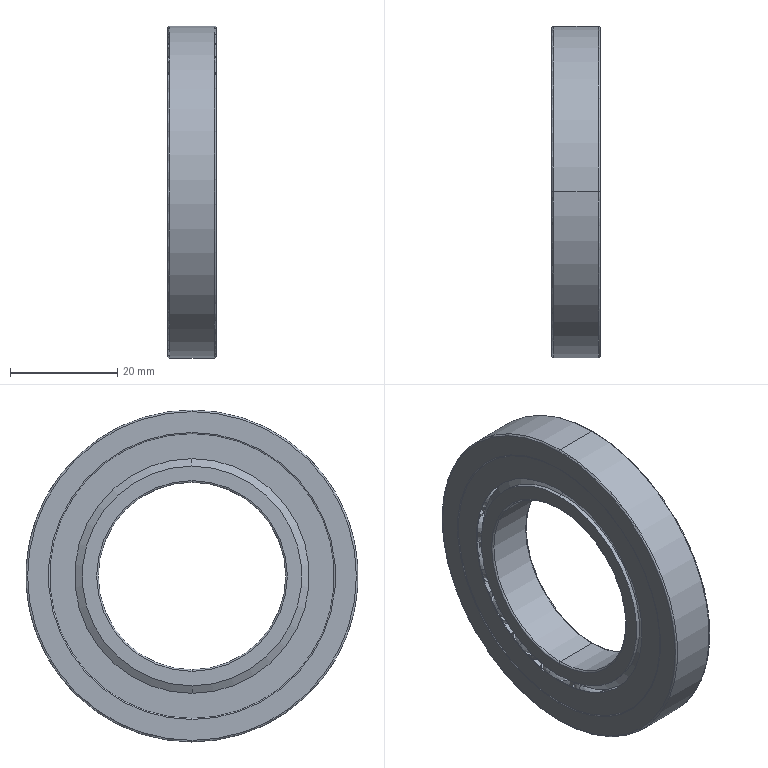Part | SolidWorks | features Revolution 5, CirPattern 2, RefAxis 1, RevCut 1 | 20 solids | 228 faces | box 9 x 62 x 62 mm | volume 14273 mm3 | cylinder 82 | sphere 76 | plane 44 | torus 22 | cone 4 | commonest cylinder face diameters 47.15 x35 49.85 x35 41 x4 53 x4 35 x2 62 x2